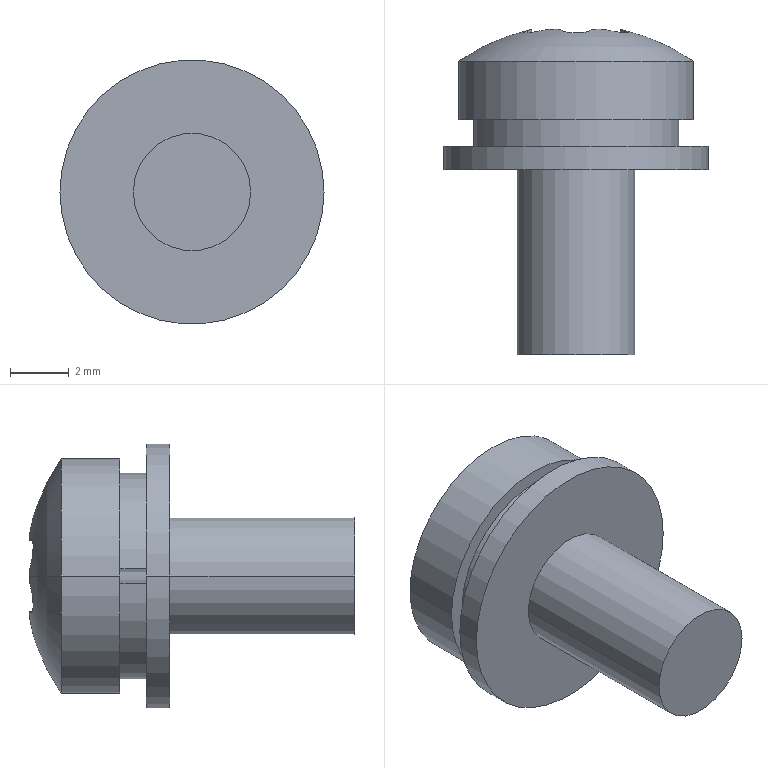Part | STEP file | LIB_68343097_M4X8 | 1 solid | 29 faces | box 9 x 11.088 x 9 mm | volume 282.702 mm3 | cylinder 20 | plane 7 | sphere 2 | commonest cylinder face diameters 0.992 x6 1.2 x6 4 x3 8 x2 9 x2 7 x1